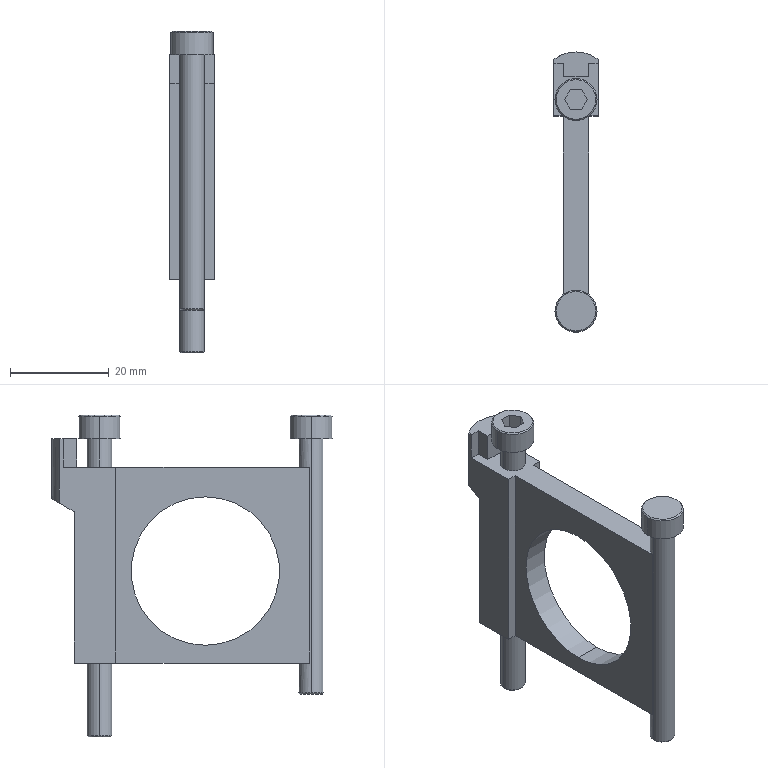Part | STEP file | AC40-04-KSTV-38JNR_AC3009A Spacer Interface | 1 solid | 52 faces | box 9 x 56.65 x 65 mm | volume 9428 mm3 | plane 31 | cylinder 13 | cone 8 | commonest cylinder face diameters 5 x6 8.5 x4 30 x2 15 x1